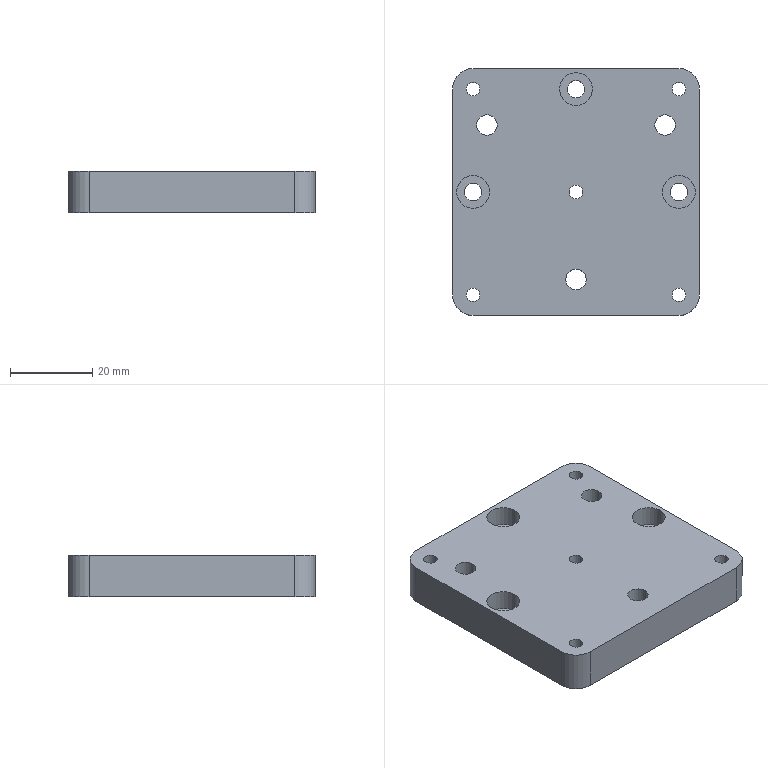Part | SolidWorks | features HoleWzd 3, Cut 1, Extrusion 1, Fillet 1, ICE 1 | 1 solid | 41 faces | box 60 x 60 x 10 mm | volume 33807 mm3 | cylinder 32 | plane 9 | commonest cylinder face diameters 3.3 x10 4.2 x6 5 x6 8 x6 10 x4
STEP:
#1=CARTESIAN_POINT('',(7.514,0.,0.));
#2=VERTEX_POINT('',#1);
#3=CARTESIAN_POINT('',(10.814,0.,0.));
#4=VERTEX_POINT('',#3);
#5=CARTESIAN_POINT('',(9.164,0.,0.));
#6=DIRECTION('',(0.,0.,1.));
#7=DIRECTION('',(1.,0.,0.));
#8=AXIS2_PLACEMENT_3D('',#5,#6,#7);
#9=CIRCLE('',#8,1.65);
#10=EDGE_CURVE('',#2,#4,#9,.T.);
#11=ORIENTED_EDGE('',*,*,#10,.F.);
#12=CARTESIAN_POINT('',(7.514,0.,10.));
#13=VERTEX_POINT('',#12);
#14=CARTESIAN_POINT('',(7.514,0.,10.));
#15=DIRECTION('',(0.,0.,1.));
#16=VECTOR('',#15,1000.);
#17=LINE('',#14,#16);
#18=EDGE_CURVE('',#2,#13,#17,.T.);
#19=ORIENTED_EDGE('',*,*,#18,.T.);
#20=CARTESIAN_POINT('',(10.814,0.,10.));
#21=VERTEX_POINT('',#20);
#22=CARTESIAN_POINT('',(9.164,0.,10.));
#23=DIRECTION('',(0.,0.,1.));
#24=DIRECTION('',(1.,0.,0.));
#25=AXIS2_PLACEMENT_3D('',#22,#23,#24);
#26=CIRCLE('',#25,1.65);
#27=EDGE_CURVE('',#13,#21,#26,.T.);
#28=ORIENTED_EDGE('',*,*,#27,.T.);
#29=CARTESIAN_POINT('',(10.814,0.,10.));
#30=DIRECTION('',(0.,0.,1.));
#31=VECTOR('',#30,1000.);
#32=LINE('',#29,#31);
#33=EDGE_CURVE('',#4,#21,#32,.T.);
#34=ORIENTED_EDGE('',*,*,#33,.F.);
#35=EDGE_LOOP('',(#11,#19,#28,#34));
#36=FACE_OUTER_BOUND('',#35,.T.);
#37=CARTESIAN_POINT('',(9.164,0.,10.));
#38=DIRECTION('',(0.,0.,1.));
#39=DIRECTION('',(1.,0.,0.));
#40=AXIS2_PLACEMENT_3D('',#37,#38,#39);
#41=CYLINDRICAL_SURFACE('',#40,1.65);
#42=ADVANCED_FACE('',(#36),#41,.F.);
#43=CARTESIAN_POINT('',(-17.486,-25.,0.));
#44=VERTEX_POINT('',#43);
#45=CARTESIAN_POINT('',(-14.186,-25.,0.));
#46=VERTEX_POINT('',#45);
#47=CARTESIAN_POINT('',(-15.836,-25.,0.));
#48=DIRECTION('',(0.,0.,1.));
#49=DIRECTION('',(1.,0.,0.));
#50=AXIS2_PLACEMENT_3D('',#47,#48,#49);
#51=CIRCLE('',#50,1.65);
#52=EDGE_CURVE('',#44,#46,#51,.T.);
#53=ORIENTED_EDGE('',*,*,#52,.F.);
#54=CARTESIAN_POINT('',(-17.486,-25.,10.));
#55=VERTEX_POINT('',#54);
#56=CARTESIAN_POINT('',(-17.486,-25.,10.));
#57=DIRECTION('',(0.,0.,1.));
#58=VECTOR('',#57,1000.);
#59=LINE('',#56,#58);
#60=EDGE_CURVE('',#44,#55,#59,.T.);
#61=ORIENTED_EDGE('',*,*,#60,.T.);
#62=CARTESIAN_POINT('',(-14.186,-25.,10.));
#63=VERTEX_POINT('',#62);
#64=CARTESIAN_POINT('',(-15.836,-25.,10.));
#65=DIRECTION('',(0.,0.,1.));
#66=DIRECTION('',(1.,0.,0.));
#67=AXIS2_PLACEMENT_3D('',#64,#65,#66);
#68=CIRCLE('',#67,1.65);
#69=EDGE_CURVE('',#55,#63,#68,.T.);
#70=ORIENTED_EDGE('',*,*,#69,.T.);
#71=CARTESIAN_POINT('',(-14.186,-25.,10.));
#72=DIRECTION('',(0.,0.,1.));
#73=VECTOR('',#72,1000.);
#74=LINE('',#71,#73);
#75=EDGE_CURVE('',#46,#63,#74,.T.);
#76=ORIENTED_EDGE('',*,*,#75,.F.);
#77=EDGE_LOOP('',(#53,#61,#70,#76));
#78=FACE_OUTER_BOUND('',#77,.T.);
#79=CARTESIAN_POINT('',(-15.836,-25.,10.));
#80=DIRECTION('',(0.,0.,1.));
#81=DIRECTION('',(1.,0.,0.));
#82=AXIS2_PLACEMENT_3D('',#79,#80,#81);
#83=CYLINDRICAL_SURFACE('',#82,1.65);
#84=ADVANCED_FACE('',(#78),#83,.F.);
#85=CARTESIAN_POINT('',(32.514,-25.,0.));
#86=VERTEX_POINT('',#85);
#87=CARTESIAN_POINT('',(35.814,-25.,0.));
#88=VERTEX_POINT('',#87);
#89=CARTESIAN_POINT('',(34.164,-25.,0.));
#90=DIRECTION('',(0.,0.,1.));
#91=DIRECTION('',(1.,0.,0.));
#92=AXIS2_PLACEMENT_3D('',#89,#90,#91);
#93=CIRCLE('',#92,1.65);
#94=EDGE_CURVE('',#86,#88,#93,.T.);
#95=ORIENTED_EDGE('',*,*,#94,.F.);
#96=CARTESIAN_POINT('',(32.514,-25.,10.));
#97=VERTEX_POINT('',#96);
#98=CARTESIAN_POINT('',(32.514,-25.,10.));
#99=DIRECTION('',(0.,0.,1.));
#100=VECTOR('',#99,1000.);
#101=LINE('',#98,#100);
#102=EDGE_CURVE('',#86,#97,#101,.T.);
#103=ORIENTED_EDGE('',*,*,#102,.T.);
#104=CARTESIAN_POINT('',(35.814,-25.,10.));
#105=VERTEX_POINT('',#104);
#106=CARTESIAN_POINT('',(34.164,-25.,10.));
#107=DIRECTION('',(0.,0.,1.));
#108=DIRECTION('',(1.,0.,0.));
#109=AXIS2_PLACEMENT_3D('',#106,#107,#108);
#110=CIRCLE('',#109,1.65);
#111=EDGE_CURVE('',#97,#105,#110,.T.);
#112=ORIENTED_EDGE('',*,*,#111,.T.);
#113=CARTESIAN_POINT('',(35.814,-25.,10.));
#114=DIRECTION('',(0.,0.,1.));
#115=VECTOR('',#114,1000.);
#116=LINE('',#113,#115);
#117=EDGE_CURVE('',#88,#105,#116,.T.);
#118=ORIENTED_EDGE('',*,*,#117,.F.);
#119=EDGE_LOOP('',(#95,#103,#112,#118));
#120=FACE_OUTER_BOUND('',#119,.T.);
#121=CARTESIAN_POINT('',(34.164,-25.,10.));
#122=DIRECTION('',(0.,0.,1.));
#123=DIRECTION('',(1.,0.,0.));
#124=AXIS2_PLACEMENT_3D('',#121,#122,#123);
#125=CYLINDRICAL_SURFACE('',#124,1.65);
#126=ADVANCED_FACE('',(#120),#125,.F.);
#127=CARTESIAN_POINT('',(32.514,25.,0.));
#128=VERTEX_POINT('',#127);
#129=CARTESIAN_POINT('',(35.814,25.,0.));
#130=VERTEX_POINT('',#129);
#131=CARTESIAN_POINT('',(34.164,25.,0.));
#132=DIRECTION('',(0.,0.,1.));
#133=DIRECTION('',(1.,0.,0.));
#134=AXIS2_PLACEMENT_3D('',#131,#132,#133);
#135=CIRCLE('',#134,1.65);
#136=EDGE_CURVE('',#128,#130,#135,.T.);
#137=ORIENTED_EDGE('',*,*,#136,.F.);
#138=CARTESIAN_POINT('',(32.514,25.,10.));
#139=VERTEX_POINT('',#138);
#140=CARTESIAN_POINT('',(32.514,25.,10.));
#141=DIRECTION('',(0.,0.,1.));
#142=VECTOR('',#141,1000.);
#143=LINE('',#140,#142);
#144=EDGE_CURVE('',#128,#139,#143,.T.);
#145=ORIENTED_EDGE('',*,*,#144,.T.);
#146=CARTESIAN_POINT('',(35.814,25.,10.));
#147=VERTEX_POINT('',#146);
#148=CARTESIAN_POINT('',(34.164,25.,10.));
#149=DIRECTION('',(0.,0.,1.));
#150=DIRECTION('',(1.,0.,0.));
#151=AXIS2_PLACEMENT_3D('',#148,#149,#150);
#152=CIRCLE('',#151,1.65);
#153=EDGE_CURVE('',#139,#147,#152,.T.);
#154=ORIENTED_EDGE('',*,*,#153,.T.);
#155=CARTESIAN_POINT('',(35.814,25.,10.));
#156=DIRECTION('',(0.,0.,1.));
#157=VECTOR('',#156,1000.);
#158=LINE('',#155,#157);
#159=EDGE_CURVE('',#130,#147,#158,.T.);
#160=ORIENTED_EDGE('',*,*,#159,.F.);
#161=EDGE_LOOP('',(#137,#145,#154,#160));
#162=FACE_OUTER_BOUND('',#161,.T.);
#163=CARTESIAN_POINT('',(34.164,25.,10.));
#164=DIRECTION('',(0.,0.,1.));
#165=DIRECTION('',(1.,0.,0.));
#166=AXIS2_PLACEMENT_3D('',#163,#164,#165);
#167=CYLINDRICAL_SURFACE('',#166,1.65);
#168=ADVANCED_FACE('',(#162),#167,.F.);
#169=CARTESIAN_POINT('',(-17.486,25.,0.));
#170=VERTEX_POINT('',#169);
#171=CARTESIAN_POINT('',(-14.186,25.,0.));
#172=VERTEX_POINT('',#171);
#173=CARTESIAN_POINT('',(-15.836,25.,0.));
#174=DIRECTION('',(0.,0.,1.));
#175=DIRECTION('',(1.,0.,0.));
#176=AXIS2_PLACEMENT_3D('',#173,#174,#175);
#177=CIRCLE('',#176,1.65);
#178=EDGE_CURVE('',#170,#172,#177,.T.);
#179=ORIENTED_EDGE('',*,*,#178,.F.);
#180=CARTESIAN_POINT('',(-17.486,25.,10.));
#181=VERTEX_POINT('',#180);
#182=CARTESIAN_POINT('',(-17.486,25.,10.));
#183=DIRECTION('',(0.,0.,1.));
#184=VECTOR('',#183,1000.);
#185=LINE('',#182,#184);
#186=EDGE_CURVE('',#170,#181,#185,.T.);
#187=ORIENTED_EDGE('',*,*,#186,.T.);
#188=CARTESIAN_POINT('',(-14.186,25.,10.));
#189=VERTEX_POINT('',#188);
#190=CARTESIAN_POINT('',(-15.836,25.,10.));
#191=DIRECTION('',(0.,0.,1.));
#192=DIRECTION('',(1.,0.,0.));
#193=AXIS2_PLACEMENT_3D('',#190,#191,#192);
#194=CIRCLE('',#193,1.65);
#195=EDGE_CURVE('',#181,#189,#194,.T.);
#196=ORIENTED_EDGE('',*,*,#195,.T.);
#197=CARTESIAN_POINT('',(-14.186,25.,10.));
#198=DIRECTION('',(0.,0.,1.));
#199=VECTOR('',#198,1000.);
#200=LINE('',#197,#199);
#201=EDGE_CURVE('',#172,#189,#200,.T.);
#202=ORIENTED_EDGE('',*,*,#201,.F.);
#203=EDGE_LOOP('',(#179,#187,#196,#202));
#204=FACE_OUTER_BOUND('',#203,.T.);
#205=CARTESIAN_POINT('',(-15.836,25.,10.));
#206=DIRECTION('',(0.,0.,1.));
#207=DIRECTION('',(1.,0.,0.));
#208=AXIS2_PLACEMENT_3D('',#205,#206,#207);
#209=CYLINDRICAL_SURFACE('',#208,1.65);
#210=ADVANCED_FACE('',(#204),#209,.F.);
#211=CARTESIAN_POINT('',(-19.836,0.,5.));
#212=VERTEX_POINT('',#211);
#213=CARTESIAN_POINT('',(-11.836,0.,5.));
#214=VERTEX_POINT('',#213);
#215=CARTESIAN_POINT('',(-15.836,0.,5.));
#216=DIRECTION('',(0.,0.,1.));
#217=DIRECTION('',(1.,0.,0.));
#218=AXIS2_PLACEMENT_3D('',#215,#216,#217);
#219=CIRCLE('',#218,4.);
#220=EDGE_CURVE('',#212,#214,#219,.T.);
#221=ORIENTED_EDGE('',*,*,#220,.F.);
#222=CARTESIAN_POINT('',(-19.836,0.,10.));
#223=VERTEX_POINT('',#222);
#224=CARTESIAN_POINT('',(-19.836,0.,5.));
#225=DIRECTION('',(0.,0.,1.));
#226=VECTOR('',#225,1000.);
#227=LINE('',#224,#226);
#228=EDGE_CURVE('',#212,#223,#227,.T.);
#229=ORIENTED_EDGE('',*,*,#228,.T.);
#230=CARTESIAN_POINT('',(-11.836,0.,10.));
#231=VERTEX_POINT('',#230);
#232=CARTESIAN_POINT('',(-15.836,0.,10.));
#233=DIRECTION('',(0.,0.,1.));
#234=DIRECTION('',(1.,0.,0.));
#235=AXIS2_PLACEMENT_3D('',#232,#233,#234);
#236=CIRCLE('',#235,4.);
#237=EDGE_CURVE('',#223,#231,#236,.T.);
#238=ORIENTED_EDGE('',*,*,#237,.T.);
#239=CARTESIAN_POINT('',(-11.836,0.,5.));
#240=DIRECTION('',(0.,0.,1.));
#241=VECTOR('',#240,1000.);
#242=LINE('',#239,#241);
#243=EDGE_CURVE('',#214,#231,#242,.T.);
#244=ORIENTED_EDGE('',*,*,#243,.F.);
#245=EDGE_LOOP('',(#221,#229,#238,#244));
#246=FACE_OUTER_BOUND('',#245,.T.);
#247=CARTESIAN_POINT('',(-15.836,0.,5.));
#248=DIRECTION('',(0.,0.,1.));
#249=DIRECTION('',(1.,0.,0.));
#250=AXIS2_PLACEMENT_3D('',#247,#248,#249);
#251=CYLINDRICAL_SURFACE('',#250,4.);
#252=ADVANCED_FACE('',(#246),#251,.F.);
#253=CARTESIAN_POINT('',(30.164,0.,5.));
#254=VERTEX_POINT('',#253);
#255=CARTESIAN_POINT('',(38.164,0.,5.));
#256=VERTEX_POINT('',#255);
#257=CARTESIAN_POINT('',(34.164,0.,5.));
#258=DIRECTION('',(0.,0.,1.));
#259=DIRECTION('',(1.,0.,0.));
#260=AXIS2_PLACEMENT_3D('',#257,#258,#259);
#261=CIRCLE('',#260,4.);
#262=EDGE_CURVE('',#254,#256,#261,.T.);
#263=ORIENTED_EDGE('',*,*,#262,.F.);
#264=CARTESIAN_POINT('',(30.164,0.,10.));
#265=VERTEX_POINT('',#264);
#266=CARTESIAN_POINT('',(30.164,0.,5.));
#267=DIRECTION('',(0.,0.,1.));
#268=VECTOR('',#267,1000.);
#269=LINE('',#266,#268);
#270=EDGE_CURVE('',#254,#265,#269,.T.);
#271=ORIENTED_EDGE('',*,*,#270,.T.);
#272=CARTESIAN_POINT('',(38.164,0.,10.));
#273=VERTEX_POINT('',#272);
#274=CARTESIAN_POINT('',(34.164,0.,10.));
#275=DIRECTION('',(0.,0.,1.));
#276=DIRECTION('',(1.,0.,0.));
#277=AXIS2_PLACEMENT_3D('',#274,#275,#276);
#278=CIRCLE('',#277,4.);
#279=EDGE_CURVE('',#265,#273,#278,.T.);
#280=ORIENTED_EDGE('',*,*,#279,.T.);
#281=CARTESIAN_POINT('',(38.164,0.,5.));
#282=DIRECTION('',(0.,0.,1.));
#283=VECTOR('',#282,1000.);
#284=LINE('',#281,#283);
#285=EDGE_CURVE('',#256,#273,#284,.T.);
#286=ORIENTED_EDGE('',*,*,#285,.F.);
#287=EDGE_LOOP('',(#263,#271,#280,#286));
#288=FACE_OUTER_BOUND('',#287,.T.);
#289=CARTESIAN_POINT('',(34.164,0.,5.));
#290=DIRECTION('',(0.,0.,1.));
#291=DIRECTION('',(1.,0.,0.));
#292=AXIS2_PLACEMENT_3D('',#289,#290,#291);
#293=CYLINDRICAL_SURFACE('',#292,4.);
#294=ADVANCED_FACE('',(#288),#293,.F.);
#295=CARTESIAN_POINT('',(5.164,25.,5.));
#296=VERTEX_POINT('',#295);
#297=CARTESIAN_POINT('',(13.164,25.,5.));
#298=VERTEX_POINT('',#297);
#299=CARTESIAN_POINT('',(9.164,25.,5.));
#300=DIRECTION('',(0.,0.,1.));
#301=DIRECTION('',(1.,0.,0.));
#302=AXIS2_PLACEMENT_3D('',#299,#300,#301);
#303=CIRCLE('',#302,4.);
#304=EDGE_CURVE('',#296,#298,#303,.T.);
#305=ORIENTED_EDGE('',*,*,#304,.F.);
#306=CARTESIAN_POINT('',(5.164,25.,10.));
#307=VERTEX_POINT('',#306);
#308=CARTESIAN_POINT('',(5.164,25.,5.));
#309=DIRECTION('',(0.,0.,1.));
#310=VECTOR('',#309,1000.);
#311=LINE('',#308,#310);
#312=EDGE_CURVE('',#296,#307,#311,.T.);
#313=ORIENTED_EDGE('',*,*,#312,.T.);
#314=CARTESIAN_POINT('',(13.164,25.,10.));
#315=VERTEX_POINT('',#314);
#316=CARTESIAN_POINT('',(9.164,25.,10.));
#317=DIRECTION('',(0.,0.,1.));
#318=DIRECTION('',(1.,0.,0.));
#319=AXIS2_PLACEMENT_3D('',#316,#317,#318);
#320=CIRCLE('',#319,4.);
#321=EDGE_CURVE('',#307,#315,#320,.T.);
#322=ORIENTED_EDGE('',*,*,#321,.T.);
#323=CARTESIAN_POINT('',(13.164,25.,5.));
#324=DIRECTION('',(0.,0.,1.));
#325=VECTOR('',#324,1000.);
#326=LINE('',#323,#325);
#327=EDGE_CURVE('',#298,#315,#326,.T.);
#328=ORIENTED_EDGE('',*,*,#327,.F.);
#329=EDGE_LOOP('',(#305,#313,#322,#328));
#330=FACE_OUTER_BOUND('',#329,.T.);
#331=CARTESIAN_POINT('',(9.164,25.,5.));
#332=DIRECTION('',(0.,0.,1.));
#333=DIRECTION('',(1.,0.,0.));
#334=AXIS2_PLACEMENT_3D('',#331,#332,#333);
#335=CYLINDRICAL_SURFACE('',#334,4.);
#336=ADVANCED_FACE('',(#330),#335,.F.);
#337=CARTESIAN_POINT('',(6.664,-21.25,0.));
#338=VERTEX_POINT('',#337);
#339=CARTESIAN_POINT('',(11.664,-21.25,0.));
#340=VERTEX_POINT('',#339);
#341=CARTESIAN_POINT('',(9.164,-21.25,0.));
#342=DIRECTION('',(0.,0.,1.));
#343=DIRECTION('',(1.,0.,0.));
#344=AXIS2_PLACEMENT_3D('',#341,#342,#343);
#345=CIRCLE('',#344,2.5);
#346=EDGE_CURVE('',#338,#340,#345,.T.);
#347=ORIENTED_EDGE('',*,*,#346,.F.);
#348=CARTESIAN_POINT('',(6.664,-21.25,10.));
#349=VERTEX_POINT('',#348);
#350=CARTESIAN_POINT('',(6.664,-21.25,10.));
#351=DIRECTION('',(0.,0.,1.));
#352=VECTOR('',#351,1000.);
#353=LINE('',#350,#352);
#354=EDGE_CURVE('',#338,#349,#353,.T.);
#355=ORIENTED_EDGE('',*,*,#354,.T.);
#356=CARTESIAN_POINT('',(11.664,-21.25,10.));
#357=VERTEX_POINT('',#356);
#358=CARTESIAN_POINT('',(9.164,-21.25,10.));
#359=DIRECTION('',(0.,0.,1.));
#360=DIRECTION('',(1.,0.,0.));
#361=AXIS2_PLACEMENT_3D('',#358,#359,#360);
#362=CIRCLE('',#361,2.5);
#363=EDGE_CURVE('',#349,#357,#362,.T.);
#364=ORIENTED_EDGE('',*,*,#363,.T.);
#365=CARTESIAN_POINT('',(11.664,-21.25,10.));
#366=DIRECTION('',(0.,0.,1.));
#367=VECTOR('',#366,1000.);
#368=LINE('',#365,#367);
#369=EDGE_CURVE('',#340,#357,#368,.T.);
#370=ORIENTED_EDGE('',*,*,#369,.F.);
#371=EDGE_LOOP('',(#347,#355,#364,#370));
#372=FACE_OUTER_BOUND('',#371,.T.);
#373=CARTESIAN_POINT('',(9.164,-21.25,10.));
#374=DIRECTION('',(0.,0.,1.));
#375=DIRECTION('',(1.,0.,0.));
#376=AXIS2_PLACEMENT_3D('',#373,#374,#375);
#377=CYLINDRICAL_SURFACE('',#376,2.5);
#378=ADVANCED_FACE('',(#372),#377,.F.);
#379=CARTESIAN_POINT('',(28.314,16.25,0.));
#380=VERTEX_POINT('',#379);
#381=CARTESIAN_POINT('',(33.314,16.25,0.));
#382=VERTEX_POINT('',#381);
#383=CARTESIAN_POINT('',(30.814,16.25,0.));
#384=DIRECTION('',(0.,0.,1.));
#385=DIRECTION('',(1.,0.,0.));
#386=AXIS2_PLACEMENT_3D('',#383,#384,#385);
#387=CIRCLE('',#386,2.5);
#388=EDGE_CURVE('',#380,#382,#387,.T.);
#389=ORIENTED_EDGE('',*,*,#388,.F.);
#390=CARTESIAN_POINT('',(28.314,16.25,10.));
#391=VERTEX_POINT('',#390);
#392=CARTESIAN_POINT('',(28.314,16.25,10.));
#393=DIRECTION('',(0.,0.,1.));
#394=VECTOR('',#393,1000.);
#395=LINE('',#392,#394);
#396=EDGE_CURVE('',#380,#391,#395,.T.);
#397=ORIENTED_EDGE('',*,*,#396,.T.);
#398=CARTESIAN_POINT('',(33.314,16.25,10.));
#399=VERTEX_POINT('',#398);
#400=CARTESIAN_POINT('',(30.814,16.25,10.));
#401=DIRECTION('',(0.,0.,1.));
#402=DIRECTION('',(1.,0.,0.));
#403=AXIS2_PLACEMENT_3D('',#400,#401,#402);
#404=CIRCLE('',#403,2.5);
#405=EDGE_CURVE('',#391,#399,#404,.T.);
#406=ORIENTED_EDGE('',*,*,#405,.T.);
#407=CARTESIAN_POINT('',(33.314,16.25,10.));
#408=DIRECTION('',(0.,0.,1.));
#409=VECTOR('',#408,1000.);
#410=LINE('',#407,#409);
#411=EDGE_CURVE('',#382,#399,#410,.T.);
#412=ORIENTED_EDGE('',*,*,#411,.F.);
#413=EDGE_LOOP('',(#389,#397,#406,#412));
#414=FACE_OUTER_BOUND('',#413,.T.);
#415=CARTESIAN_POINT('',(30.814,16.25,10.));
#416=DIRECTION('',(0.,0.,1.));
#417=DIRECTION('',(1.,0.,0.));
#418=AXIS2_PLACEMENT_3D('',#415,#416,#417);
#419=CYLINDRICAL_SURFACE('',#418,2.5);
#420=ADVANCED_FACE('',(#414),#419,.F.);
#421=CARTESIAN_POINT('',(-14.987,16.25,0.));
#422=VERTEX_POINT('',#421);
#423=CARTESIAN_POINT('',(-9.987,16.25,0.));
#424=VERTEX_POINT('',#423);
#425=CARTESIAN_POINT('',(-12.487,16.25,0.));
#426=DIRECTION('',(0.,0.,1.));
#427=DIRECTION('',(1.,0.,0.));
#428=AXIS2_PLACEMENT_3D('',#425,#426,#427);
#429=CIRCLE('',#428,2.5);
#430=EDGE_CURVE('',#422,#424,#429,.T.);
#431=ORIENTED_EDGE('',*,*,#430,.F.);
#432=CARTESIAN_POINT('',(-14.987,16.25,10.));
#433=VERTEX_POINT('',#432);
#434=CARTESIAN_POINT('',(-14.987,16.25,10.));
#435=DIRECTION('',(0.,0.,1.));
#436=VECTOR('',#435,1000.);
#437=LINE('',#434,#436);
#438=EDGE_CURVE('',#422,#433,#437,.T.);
#439=ORIENTED_EDGE('',*,*,#438,.T.);
#440=CARTESIAN_POINT('',(-9.987,16.25,10.));
#441=VERTEX_POINT('',#440);
#442=CARTESIAN_POINT('',(-12.487,16.25,10.));
#443=DIRECTION('',(0.,0.,1.));
#444=DIRECTION('',(1.,0.,0.));
#445=AXIS2_PLACEMENT_3D('',#442,#443,#444);
#446=CIRCLE('',#445,2.5);
#447=EDGE_CURVE('',#433,#441,#446,.T.);
#448=ORIENTED_EDGE('',*,*,#447,.T.);
#449=CARTESIAN_POINT('',(-9.987,16.25,10.));
#450=DIRECTION('',(0.,0.,1.));
#451=VECTOR('',#450,1000.);
#452=LINE('',#449,#451);
#453=EDGE_CURVE('',#424,#441,#452,.T.);
#454=ORIENTED_EDGE('',*,*,#453,.F.);
#455=EDGE_LOOP('',(#431,#439,#448,#454));
#456=FACE_OUTER_BOUND('',#455,.T.);
#457=CARTESIAN_POINT('',(-12.487,16.25,10.));
#458=DIRECTION('',(0.,0.,1.));
#459=DIRECTION('',(1.,0.,0.));
#460=AXIS2_PLACEMENT_3D('',#457,#458,#459);
#461=CYLINDRICAL_SURFACE('',#460,2.5);
#462=ADVANCED_FACE('',(#456),#461,.F.);
#463=CARTESIAN_POINT('',(7.064,25.,0.));
#464=VERTEX_POINT('',#463);
#465=CARTESIAN_POINT('',(11.264,25.,0.));
#466=VERTEX_POINT('',#465);
#467=CARTESIAN_POINT('',(9.164,25.,0.));
#468=DIRECTION('',(0.,0.,1.));
#469=DIRECTION('',(1.,0.,0.));
#470=AXIS2_PLACEMENT_3D('',#467,#468,#469);
#471=CIRCLE('',#470,2.1);
#472=EDGE_CURVE('',#464,#466,#471,.T.);
#473=ORIENTED_EDGE('',*,*,#472,.F.);
#474=CARTESIAN_POINT('',(7.064,25.,5.));
#475=VERTEX_POINT('',#474);
#476=CARTESIAN_POINT('',(7.064,25.,0.));
#477=DIRECTION('',(0.,0.,1.));
#478=VECTOR('',#477,1000.);
#479=LINE('',#476,#478);
#480=EDGE_CURVE('',#464,#475,#479,.T.);
#481=ORIENTED_EDGE('',*,*,#480,.T.);
#482=CARTESIAN_POINT('',(11.264,25.,5.));
#483=VERTEX_POINT('',#482);
#484=CARTESIAN_POINT('',(9.164,25.,5.));
#485=DIRECTION('',(0.,0.,-1.));
#486=DIRECTION('',(1.,0.,0.));
#487=AXIS2_PLACEMENT_3D('',#484,#485,#486);
#488=CIRCLE('',#487,2.1);
#489=EDGE_CURVE('',#483,#475,#488,.T.);
#490=ORIENTED_EDGE('',*,*,#489,.F.);
#491=CARTESIAN_POINT('',(11.264,25.,0.));
#492=DIRECTION('',(0.,0.,1.));
#493=VECTOR('',#492,1000.);
#494=LINE('',#491,#493);
#495=EDGE_CURVE('',#466,#483,#494,.T.);
#496=ORIENTED_EDGE('',*,*,#495,.F.);
#497=EDGE_LOOP('',(#473,#481,#490,#496));
#498=FACE_OUTER_BOUND('',#497,.T.);
#499=CARTESIAN_POINT('',(9.164,25.,0.));
#500=DIRECTION('',(0.,0.,1.));
#501=DIRECTION('',(1.,0.,0.));
#502=AXIS2_PLACEMENT_3D('',#499,#500,#501);
#503=CYLINDRICAL_SURFACE('',#502,2.1);
#504=ADVANCED_FACE('',(#498),#503,.F.);
#505=CARTESIAN_POINT('',(32.064,0.,0.));
#506=VERTEX_POINT('',#505);
#507=CARTESIAN_POINT('',(36.264,0.,0.));
#508=VERTEX_POINT('',#507);
#509=CARTESIAN_POINT('',(34.164,0.,0.));
#510=DIRECTION('',(0.,0.,1.));
#511=DIRECTION('',(1.,0.,0.));
#512=AXIS2_PLACEMENT_3D('',#509,#510,#511);
#513=CIRCLE('',#512,2.1);
#514=EDGE_CURVE('',#506,#508,#513,.T.);
#515=ORIENTED_EDGE('',*,*,#514,.F.);
#516=CARTESIAN_POINT('',(32.064,0.,5.));
#517=VERTEX_POINT('',#516);
#518=CARTESIAN_POINT('',(32.064,0.,0.));
#519=DIRECTION('',(0.,0.,1.));
#520=VECTOR('',#519,1000.);
#521=LINE('',#518,#520);
#522=EDGE_CURVE('',#506,#517,#521,.T.);
#523=ORIENTED_EDGE('',*,*,#522,.T.);
#524=CARTESIAN_POINT('',(36.264,0.,5.));
#525=VERTEX_POINT('',#524);
#526=CARTESIAN_POINT('',(34.164,0.,5.));
#527=DIRECTION('',(0.,0.,-1.));
#528=DIRECTION('',(1.,0.,0.));
#529=AXIS2_PLACEMENT_3D('',#526,#527,#528);
#530=CIRCLE('',#529,2.1);
#531=EDGE_CURVE('',#525,#517,#530,.T.);
#532=ORIENTED_EDGE('',*,*,#531,.F.);
#533=CARTESIAN_POINT('',(36.264,0.,0.));
#534=DIRECTION('',(0.,0.,1.));
#535=VECTOR('',#534,1000.);
#536=LINE('',#533,#535);
#537=EDGE_CURVE('',#508,#525,#536,.T.);
#538=ORIENTED_EDGE('',*,*,#537,.F.);
#539=EDGE_LOOP('',(#515,#523,#532,#538));
#540=FACE_OUTER_BOUND('',#539,.T.);
#541=CARTESIAN_POINT('',(34.164,0.,0.));
#542=DIRECTION('',(0.,0.,1.));
#543=DIRECTION('',(1.,0.,0.));
#544=AXIS2_PLACEMENT_3D('',#541,#542,#543);
#545=CYLINDRICAL_SURFACE('',#544,2.1);
#546=ADVANCED_FACE('',(#540),#545,.F.);
#547=CARTESIAN_POINT('',(-17.936,0.,0.));
#548=VERTEX_POINT('',#547);
#549=CARTESIAN_POINT('',(-13.736,0.,0.));
#550=VERTEX_POINT('',#549);
#551=CARTESIAN_POINT('',(-15.836,0.,0.));
#552=DIRECTION('',(0.,0.,1.));
#553=DIRECTION('',(1.,0.,0.));
#554=AXIS2_PLACEMENT_3D('',#551,#552,#553);
#555=CIRCLE('',#554,2.1);
#556=EDGE_CURVE('',#548,#550,#555,.T.);
#557=ORIENTED_EDGE('',*,*,#556,.F.);
#558=CARTESIAN_POINT('',(-17.936,0.,5.));
#559=VERTEX_POINT('',#558);
#560=CARTESIAN_POINT('',(-17.936,0.,0.));
#561=DIRECTION('',(0.,0.,1.));
#562=VECTOR('',#561,1000.);
#563=LINE('',#560,#562);
#564=EDGE_CURVE('',#548,#559,#563,.T.);
#565=ORIENTED_EDGE('',*,*,#564,.T.);
#566=CARTESIAN_POINT('',(-13.736,0.,5.));
#567=VERTEX_POINT('',#566);
#568=CARTESIAN_POINT('',(-15.836,0.,5.));
#569=DIRECTION('',(0.,0.,-1.));
#570=DIRECTION('',(1.,0.,0.));
#571=AXIS2_PLACEMENT_3D('',#568,#569,#570);
#572=CIRCLE('',#571,2.1);
#573=EDGE_CURVE('',#567,#559,#572,.T.);
#574=ORIENTED_EDGE('',*,*,#573,.F.);
#575=CARTESIAN_POINT('',(-13.736,0.,0.));
#576=DIRECTION('',(0.,0.,1.));
#577=VECTOR('',#576,1000.);
#578=LINE('',#575,#577);
#579=EDGE_CURVE('',#550,#567,#578,.T.);
#580=ORIENTED_EDGE('',*,*,#579,.F.);
#581=EDGE_LOOP('',(#557,#565,#574,#580));
#582=FACE_OUTER_BOUND('',#581,.T.);
#583=CARTESIAN_POINT('',(-15.836,0.,0.));
#584=DIRECTION('',(0.,0.,1.));
#585=DIRECTION('',(1.,0.,0.));
#586=AXIS2_PLACEMENT_3D('',#583,#584,#585);
#587=CYLINDRICAL_SURFACE('',#586,2.1);
#588=ADVANCED_FACE('',(#582),#587,.F.);
#589=ORIENTED_EDGE('',*,*,#564,.F.);
#590=CARTESIAN_POINT('',(-15.836,0.,0.));
#591=DIRECTION('',(0.,0.,1.));
#592=DIRECTION('',(1.,0.,0.));
#593=AXIS2_PLACEMENT_3D('',#590,#591,#592);
#594=CIRCLE('',#593,2.1);
#595=EDGE_CURVE('',#550,#548,#594,.T.);
#596=ORIENTED_EDGE('',*,*,#595,.F.);
#597=ORIENTED_EDGE('',*,*,#579,.T.);
#598=CARTESIAN_POINT('',(-15.836,0.,5.));
#599=DIRECTION('',(0.,0.,-1.));
#600=DIRECTION('',(1.,0.,0.));
#601=AXIS2_PLACEMENT_3D('',#598,#599,#600);
#602=CIRCLE('',#601,2.1);
#603=EDGE_CURVE('',#559,#567,#602,.T.);
#604=ORIENTED_EDGE('',*,*,#603,.F.);
#605=EDGE_LOOP('',(#589,#596,#597,#604));
#606=FACE_OUTER_BOUND('',#605,.T.);
#607=CARTESIAN_POINT('',(-15.836,0.,0.));
#608=DIRECTION('',(0.,0.,1.));
#609=DIRECTION('',(1.,0.,0.));
#610=AXIS2_PLACEMENT_3D('',#607,#608,#609);
#611=CYLINDRICAL_SURFACE('',#610,2.1);
#612=ADVANCED_FACE('',(#606),#611,.F.);
#613=ORIENTED_EDGE('',*,*,#522,.F.);
#614=CARTESIAN_POINT('',(34.164,0.,0.));
#615=DIRECTION('',(0.,0.,1.));
#616=DIRECTION('',(1.,0.,0.));
#617=AXIS2_PLACEMENT_3D('',#614,#615,#616);
#618=CIRCLE('',#617,2.1);
#619=EDGE_CURVE('',#508,#506,#618,.T.);
#620=ORIENTED_EDGE('',*,*,#619,.F.);
#621=ORIENTED_EDGE('',*,*,#537,.T.);
#622=CARTESIAN_POINT('',(34.164,0.,5.));
#623=DIRECTION('',(0.,0.,-1.));
#624=DIRECTION('',(1.,0.,0.));
#625=AXIS2_PLACEMENT_3D('',#622,#623,#624);
#626=CIRCLE('',#625,2.1);
#627=EDGE_CURVE('',#517,#525,#626,.T.);
#628=ORIENTED_EDGE('',*,*,#627,.F.);
#629=EDGE_LOOP('',(#613,#620,#621,#628));
#630=FACE_OUTER_BOUND('',#629,.T.);
#631=CARTESIAN_POINT('',(34.164,0.,0.));
#632=DIRECTION('',(0.,0.,1.));
#633=DIRECTION('',(1.,0.,0.));
#634=AXIS2_PLACEMENT_3D('',#631,#632,#633);
#635=CYLINDRICAL_SURFACE('',#634,2.1);
#636=ADVANCED_FACE('',(#630),#635,.F.);
#637=ORIENTED_EDGE('',*,*,#480,.F.);
#638=CARTESIAN_POINT('',(9.164,25.,0.));
#639=DIRECTION('',(0.,0.,1.));
#640=DIRECTION('',(1.,0.,0.));
#641=AXIS2_PLACEMENT_3D('',#638,#639,#640);
#642=CIRCLE('',#641,2.1);
#643=EDGE_CURVE('',#466,#464,#642,.T.);
#644=ORIENTED_EDGE('',*,*,#643,.F.);
#645=ORIENTED_EDGE('',*,*,#495,.T.);
#646=CARTESIAN_POINT('',(9.164,25.,5.));
#647=DIRECTION('',(0.,0.,-1.));
#648=DIRECTION('',(1.,0.,0.));
#649=AXIS2_PLACEMENT_3D('',#646,#647,#648);
#650=CIRCLE('',#649,2.1);
#651=EDGE_CURVE('',#475,#483,#650,.T.);
#652=ORIENTED_EDGE('',*,*,#651,.F.);
#653=EDGE_LOOP('',(#637,#644,#645,#652));
#654=FACE_OUTER_BOUND('',#653,.T.);
#655=CARTESIAN_POINT('',(9.164,25.,0.));
#656=DIRECTION('',(0.,0.,1.));
#657=DIRECTION('',(1.,0.,0.));
#658=AXIS2_PLACEMENT_3D('',#655,#656,#657);
#659=CYLINDRICAL_SURFACE('',#658,2.1);
#660=ADVANCED_FACE('',(#654),#659,.F.);
#661=CARTESIAN_POINT('',(-20.836,25.,10.));
#662=VERTEX_POINT('',#661);
#663=CARTESIAN_POINT('',(-20.836,-25.,10.));
#664=VERTEX_POINT('',#663);
#665=CARTESIAN_POINT('',(-20.836,-30.,10.));
#666=DIRECTION('',(0.,-1.,0.));
#667=VECTOR('',#666,1000.);
#668=LINE('',#665,#667);
#669=EDGE_CURVE('',#662,#664,#668,.T.);
#670=ORIENTED_EDGE('',*,*,#669,.F.);
#671=CARTESIAN_POINT('',(-20.836,25.,0.));
#672=VERTEX_POINT('',#671);
#673=CARTESIAN_POINT('',(-20.836,25.,10.));
#674=DIRECTION('',(0.,0.,-1.));
#675=VECTOR('',#674,1000.);
#676=LINE('',#673,#675);
#677=EDGE_CURVE('',#662,#672,#676,.T.);
#678=ORIENTED_EDGE('',*,*,#677,.T.);
#679=CARTESIAN_POINT('',(-20.836,-25.,0.));
#680=VERTEX_POINT('',#679);
#681=CARTESIAN_POINT('',(-20.836,-30.,0.));
#682=DIRECTION('',(0.,-1.,0.));
#683=VECTOR('',#682,1000.);
#684=LINE('',#681,#683);
#685=EDGE_CURVE('',#672,#680,#684,.T.);
#686=ORIENTED_EDGE('',*,*,#685,.T.);
#687=CARTESIAN_POINT('',(-20.836,-25.,10.));
#688=DIRECTION('',(0.,0.,1.));
#689=VECTOR('',#688,1000.);
#690=LINE('',#687,#689);
#691=EDGE_CURVE('',#680,#664,#690,.T.);
#692=ORIENTED_EDGE('',*,*,#691,.T.);
#693=EDGE_LOOP('',(#670,#678,#686,#692));
#694=FACE_OUTER_BOUND('',#693,.T.);
#695=CARTESIAN_POINT('',(-20.836,-30.,10.));
#696=DIRECTION('',(1.,0.,0.));
#697=DIRECTION('',(0.,0.,-1.));
#698=AXIS2_PLACEMENT_3D('',#695,#696,#697);
#699=PLANE('',#698);
#700=ADVANCED_FACE('',(#694),#699,.F.);
#701=CARTESIAN_POINT('',(-15.836,-30.,0.));
#702=VERTEX_POINT('',#701);
#703=CARTESIAN_POINT('',(34.164,-30.,0.));
#704=VERTEX_POINT('',#703);
#705=CARTESIAN_POINT('',(39.164,-30.,0.));
#706=DIRECTION('',(1.,0.,0.));
#707=VECTOR('',#706,1000.);
#708=LINE('',#705,#707);
#709=EDGE_CURVE('',#702,#704,#708,.T.);
#710=ORIENTED_EDGE('',*,*,#709,.T.);
#711=CARTESIAN_POINT('',(34.164,-30.,10.));
#712=VERTEX_POINT('',#711);
#713=CARTESIAN_POINT('',(34.164,-30.,10.));
#714=DIRECTION('',(0.,0.,1.));
#715=VECTOR('',#714,1000.);
#716=LINE('',#713,#715);
#717=EDGE_CURVE('',#704,#712,#716,.T.);
#718=ORIENTED_EDGE('',*,*,#717,.T.);
#719=CARTESIAN_POINT('',(-15.836,-30.,10.));
#720=VERTEX_POINT('',#719);
#721=CARTESIAN_POINT('',(39.164,-30.,10.));
#722=DIRECTION('',(1.,0.,0.));
#723=VECTOR('',#722,1000.);
#724=LINE('',#721,#723);
#725=EDGE_CURVE('',#720,#712,#724,.T.);
#726=ORIENTED_EDGE('',*,*,#725,.F.);
#727=CARTESIAN_POINT('',(-15.836,-30.,10.));
#728=DIRECTION('',(0.,0.,-1.));
#729=VECTOR('',#728,1000.);
#730=LINE('',#727,#729);
#731=EDGE_CURVE('',#720,#702,#730,.T.);
#732=ORIENTED_EDGE('',*,*,#731,.T.);
#733=EDGE_LOOP('',(#710,#718,#726,#732));
#734=FACE_OUTER_BOUND('',#733,.T.);
#735=CARTESIAN_POINT('',(39.164,-30.,10.));
#736=DIRECTION('',(0.,1.,0.));
#737=DIRECTION('',(-1.,0.,0.));
#738=AXIS2_PLACEMENT_3D('',#735,#736,#737);
#739=PLANE('',#738);
#740=ADVANCED_FACE('',(#734),#739,.F.);
#741=CARTESIAN_POINT('',(39.164,-25.,0.));
#742=VERTEX_POINT('',#741);
#743=CARTESIAN_POINT('',(39.164,25.,0.));
#744=VERTEX_POINT('',#743);
#745=CARTESIAN_POINT('',(39.164,-30.,0.));
#746=DIRECTION('',(0.,1.,0.));
#747=VECTOR('',#746,1000.);
#748=LINE('',#745,#747);
#749=EDGE_CURVE('',#742,#744,#748,.T.);
#750=ORIENTED_EDGE('',*,*,#749,.T.);
#751=CARTESIAN_POINT('',(39.164,25.,10.));
#752=VERTEX_POINT('',#751);
#753=CARTESIAN_POINT('',(39.164,25.,10.));
#754=DIRECTION('',(0.,0.,1.));
#755=VECTOR('',#754,1000.);
#756=LINE('',#753,#755);
#757=EDGE_CURVE('',#744,#752,#756,.T.);
#758=ORIENTED_EDGE('',*,*,#757,.T.);
#759=CARTESIAN_POINT('',(39.164,-25.,10.));
#760=VERTEX_POINT('',#759);
#761=CARTESIAN_POINT('',(39.164,-30.,10.));
#762=DIRECTION('',(0.,1.,0.));
#763=VECTOR('',#762,1000.);
#764=LINE('',#761,#763);
#765=EDGE_CURVE('',#760,#752,#764,.T.);
#766=ORIENTED_EDGE('',*,*,#765,.F.);
#767=CARTESIAN_POINT('',(39.164,-25.,10.));
#768=DIRECTION('',(0.,0.,-1.));
#769=VECTOR('',#768,1000.);
#770=LINE('',#767,#769);
#771=EDGE_CURVE('',#760,#742,#770,.T.);
#772=ORIENTED_EDGE('',*,*,#771,.T.);
#773=EDGE_LOOP('',(#750,#758,#766,#772));
#774=FACE_OUTER_BOUND('',#773,.T.);
#775=CARTESIAN_POINT('',(39.164,-30.,10.));
#776=DIRECTION('',(-1.,0.,0.));
#777=DIRECTION('',(0.,0.,1.));
#778=AXIS2_PLACEMENT_3D('',#775,#776,#777);
#779=PLANE('',#778);
#780=ADVANCED_FACE('',(#774),#779,.F.);
#781=CARTESIAN_POINT('',(34.164,30.,0.));
#782=VERTEX_POINT('',#781);
#783=CARTESIAN_POINT('',(-15.836,30.,0.));
#784=VERTEX_POINT('',#783);
#785=CARTESIAN_POINT('',(39.164,30.,0.));
#786=DIRECTION('',(-1.,0.,0.));
#787=VECTOR('',#786,1000.);
#788=LINE('',#785,#787);
#789=EDGE_CURVE('',#782,#784,#788,.T.);
#790=ORIENTED_EDGE('',*,*,#789,.T.);
#791=CARTESIAN_POINT('',(-15.836,30.,10.));
#792=VERTEX_POINT('',#791);
#793=CARTESIAN_POINT('',(-15.836,30.,10.));
#794=DIRECTION('',(0.,0.,1.));
#795=VECTOR('',#794,1000.);
#796=LINE('',#793,#795);
#797=EDGE_CURVE('',#784,#792,#796,.T.);
#798=ORIENTED_EDGE('',*,*,#797,.T.);
#799=CARTESIAN_POINT('',(34.164,30.,10.));
#800=VERTEX_POINT('',#799);
#801=CARTESIAN_POINT('',(39.164,30.,10.));
#802=DIRECTION('',(-1.,0.,0.));
#803=VECTOR('',#802,1000.);
#804=LINE('',#801,#803);
#805=EDGE_CURVE('',#800,#792,#804,.T.);
#806=ORIENTED_EDGE('',*,*,#805,.F.);
#807=CARTESIAN_POINT('',(34.164,30.,10.));
#808=DIRECTION('',(0.,0.,-1.));
#809=VECTOR('',#808,1000.);
#810=LINE('',#807,#809);
#811=EDGE_CURVE('',#800,#782,#810,.T.);
#812=ORIENTED_EDGE('',*,*,#811,.T.);
#813=EDGE_LOOP('',(#790,#798,#806,#812));
#814=FACE_OUTER_BOUND('',#813,.T.);
#815=CARTESIAN_POINT('',(39.164,30.,10.));
#816=DIRECTION('',(0.,-1.,0.));
#817=DIRECTION('',(1.,0.,0.));
#818=AXIS2_PLACEMENT_3D('',#815,#816,#817);
#819=PLANE('',#818);
#820=ADVANCED_FACE('',(#814),#819,.F.);
#821=CARTESIAN_POINT('',(9.164,0.,10.));
#822=DIRECTION('',(0.,0.,1.));
#823=DIRECTION('',(1.,0.,0.));
#824=AXIS2_PLACEMENT_3D('',#821,#822,#823);
#825=CIRCLE('',#824,1.65);
#826=EDGE_CURVE('',#21,#13,#825,.T.);
#827=ORIENTED_EDGE('',*,*,#826,.F.);
#828=ORIENTED_EDGE('',*,*,#27,.F.);
#829=EDGE_LOOP('',(#827,#828));
#830=FACE_BOUND('',#829,.T.);
#831=CARTESIAN_POINT('',(-15.836,-25.,10.));
#832=DIRECTION('',(0.,0.,1.));
#833=DIRECTION('',(1.,0.,0.));
#834=AXIS2_PLACEMENT_3D('',#831,#832,#833);
#835=CIRCLE('',#834,1.65);
#836=EDGE_CURVE('',#63,#55,#835,.T.);
#837=ORIENTED_EDGE('',*,*,#836,.F.);
#838=ORIENTED_EDGE('',*,*,#69,.F.);
#839=EDGE_LOOP('',(#837,#838));
#840=FACE_BOUND('',#839,.T.);
#841=CARTESIAN_POINT('',(34.164,-25.,10.));
#842=DIRECTION('',(0.,0.,1.));
#843=DIRECTION('',(1.,0.,0.));
#844=AXIS2_PLACEMENT_3D('',#841,#842,#843);
#845=CIRCLE('',#844,1.65);
#846=EDGE_CURVE('',#105,#97,#845,.T.);
#847=ORIENTED_EDGE('',*,*,#846,.F.);
#848=ORIENTED_EDGE('',*,*,#111,.F.);
#849=EDGE_LOOP('',(#847,#848));
#850=FACE_BOUND('',#849,.T.);
#851=CARTESIAN_POINT('',(34.164,25.,10.));
#852=DIRECTION('',(0.,0.,1.));
#853=DIRECTION('',(1.,0.,0.));
#854=AXIS2_PLACEMENT_3D('',#851,#852,#853);
#855=CIRCLE('',#854,1.65);
#856=EDGE_CURVE('',#147,#139,#855,.T.);
#857=ORIENTED_EDGE('',*,*,#856,.F.);
#858=ORIENTED_EDGE('',*,*,#153,.F.);
#859=EDGE_LOOP('',(#857,#858));
#860=FACE_BOUND('',#859,.T.);
#861=CARTESIAN_POINT('',(-15.836,25.,10.));
#862=DIRECTION('',(0.,0.,1.));
#863=DIRECTION('',(1.,0.,0.));
#864=AXIS2_PLACEMENT_3D('',#861,#862,#863);
#865=CIRCLE('',#864,1.65);
#866=EDGE_CURVE('',#189,#181,#865,.T.);
#867=ORIENTED_EDGE('',*,*,#866,.F.);
#868=ORIENTED_EDGE('',*,*,#195,.F.);
#869=EDGE_LOOP('',(#867,#868));
#870=FACE_BOUND('',#869,.T.);
#871=CARTESIAN_POINT('',(-15.836,0.,10.));
#872=DIRECTION('',(0.,0.,1.));
#873=DIRECTION('',(1.,0.,0.));
#874=AXIS2_PLACEMENT_3D('',#871,#872,#873);
#875=CIRCLE('',#874,4.);
#876=EDGE_CURVE('',#231,#223,#875,.T.);
#877=ORIENTED_EDGE('',*,*,#876,.F.);
#878=ORIENTED_EDGE('',*,*,#237,.F.);
#879=EDGE_LOOP('',(#877,#878));
#880=FACE_BOUND('',#879,.T.);
#881=CARTESIAN_POINT('',(9.164,25.,10.));
#882=DIRECTION('',(0.,0.,1.));
#883=DIRECTION('',(1.,0.,0.));
#884=AXIS2_PLACEMENT_3D('',#881,#882,#883);
#885=CIRCLE('',#884,4.);
#886=EDGE_CURVE('',#315,#307,#885,.T.);
#887=ORIENTED_EDGE('',*,*,#886,.F.);
#888=ORIENTED_EDGE('',*,*,#321,.F.);
#889=EDGE_LOOP('',(#887,#888));
#890=FACE_BOUND('',#889,.T.);
#891=CARTESIAN_POINT('',(34.164,0.,10.));
#892=DIRECTION('',(0.,0.,1.));
#893=DIRECTION('',(1.,0.,0.));
#894=AXIS2_PLACEMENT_3D('',#891,#892,#893);
#895=CIRCLE('',#894,4.);
#896=EDGE_CURVE('',#273,#265,#895,.T.);
#897=ORIENTED_EDGE('',*,*,#896,.F.);
#898=ORIENTED_EDGE('',*,*,#279,.F.);
#899=EDGE_LOOP('',(#897,#898));
#900=FACE_BOUND('',#899,.T.);
#901=CARTESIAN_POINT('',(9.164,-21.25,10.));
#902=DIRECTION('',(0.,0.,1.));
#903=DIRECTION('',(1.,0.,0.));
#904=AXIS2_PLACEMENT_3D('',#901,#902,#903);
#905=CIRCLE('',#904,2.5);
#906=EDGE_CURVE('',#357,#349,#905,.T.);
#907=ORIENTED_EDGE('',*,*,#906,.F.);
#908=ORIENTED_EDGE('',*,*,#363,.F.);
#909=EDGE_LOOP('',(#907,#908));
#910=FACE_BOUND('',#909,.T.);
#911=CARTESIAN_POINT('',(30.814,16.25,10.));
#912=DIRECTION('',(0.,0.,1.));
#913=DIRECTION('',(1.,0.,0.));
#914=AXIS2_PLACEMENT_3D('',#911,#912,#913);
#915=CIRCLE('',#914,2.5);
#916=EDGE_CURVE('',#399,#391,#915,.T.);
#917=ORIENTED_EDGE('',*,*,#916,.F.);
#918=ORIENTED_EDGE('',*,*,#405,.F.);
#919=EDGE_LOOP('',(#917,#918));
#920=FACE_BOUND('',#919,.T.);
#921=CARTESIAN_POINT('',(-12.487,16.25,10.));
#922=DIRECTION('',(0.,0.,1.));
#923=DIRECTION('',(1.,0.,0.));
#924=AXIS2_PLACEMENT_3D('',#921,#922,#923);
#925=CIRCLE('',#924,2.5);
#926=EDGE_CURVE('',#441,#433,#925,.T.);
#927=ORIENTED_EDGE('',*,*,#926,.F.);
#928=ORIENTED_EDGE('',*,*,#447,.F.);
#929=EDGE_LOOP('',(#927,#928));
#930=FACE_BOUND('',#929,.T.);
#931=ORIENTED_EDGE('',*,*,#805,.T.);
#932=CARTESIAN_POINT('',(-15.836,25.,10.));
#933=DIRECTION('',(0.,0.,1.));
#934=DIRECTION('',(1.,0.,0.));
#935=AXIS2_PLACEMENT_3D('',#932,#933,#934);
#936=CIRCLE('',#935,5.);
#937=EDGE_CURVE('',#792,#662,#936,.T.);
#938=ORIENTED_EDGE('',*,*,#937,.T.);
#939=ORIENTED_EDGE('',*,*,#669,.T.);
#940=CARTESIAN_POINT('',(-15.836,-25.,10.));
#941=DIRECTION('',(0.,0.,1.));
#942=DIRECTION('',(1.,0.,0.));
#943=AXIS2_PLACEMENT_3D('',#940,#941,#942);
#944=CIRCLE('',#943,5.);
#945=EDGE_CURVE('',#664,#720,#944,.T.);
#946=ORIENTED_EDGE('',*,*,#945,.T.);
#947=ORIENTED_EDGE('',*,*,#725,.T.);
#948=CARTESIAN_POINT('',(34.164,-25.,10.));
#949=DIRECTION('',(0.,0.,1.));
#950=DIRECTION('',(1.,0.,0.));
#951=AXIS2_PLACEMENT_3D('',#948,#949,#950);
#952=CIRCLE('',#951,5.);
#953=EDGE_CURVE('',#712,#760,#952,.T.);
#954=ORIENTED_EDGE('',*,*,#953,.T.);
#955=ORIENTED_EDGE('',*,*,#765,.T.);
#956=CARTESIAN_POINT('',(34.164,25.,10.));
#957=DIRECTION('',(0.,0.,1.));
#958=DIRECTION('',(1.,0.,0.));
#959=AXIS2_PLACEMENT_3D('',#956,#957,#958);
#960=CIRCLE('',#959,5.);
#961=EDGE_CURVE('',#752,#800,#960,.T.);
#962=ORIENTED_EDGE('',*,*,#961,.T.);
#963=EDGE_LOOP('',(#931,#938,#939,#946,#947,#954,#955,#962));
#964=FACE_OUTER_BOUND('',#963,.T.);
#965=CARTESIAN_POINT('',(0.,0.,10.));
#966=DIRECTION('',(0.,0.,1.));
#967=DIRECTION('',(1.,0.,0.));
#968=AXIS2_PLACEMENT_3D('',#965,#966,#967);
#969=PLANE('',#968);
#970=ADVANCED_FACE('',(#830,#840,#850,#860,#870,#880,#890,#900,#910,#920,#930,#964),#969,.T.);
#971=CARTESIAN_POINT('',(9.164,0.,0.));
#972=DIRECTION('',(0.,0.,1.));
#973=DIRECTION('',(1.,0.,0.));
#974=AXIS2_PLACEMENT_3D('',#971,#972,#973);
#975=CIRCLE('',#974,1.65);
#976=EDGE_CURVE('',#4,#2,#975,.T.);
#977=ORIENTED_EDGE('',*,*,#976,.T.);
#978=ORIENTED_EDGE('',*,*,#10,.T.);
#979=EDGE_LOOP('',(#977,#978));
#980=FACE_BOUND('',#979,.T.);
#981=CARTESIAN_POINT('',(-15.836,-25.,0.));
#982=DIRECTION('',(0.,0.,1.));
#983=DIRECTION('',(1.,0.,0.));
#984=AXIS2_PLACEMENT_3D('',#981,#982,#983);
#985=CIRCLE('',#984,1.65);
#986=EDGE_CURVE('',#46,#44,#985,.T.);
#987=ORIENTED_EDGE('',*,*,#986,.T.);
#988=ORIENTED_EDGE('',*,*,#52,.T.);
#989=EDGE_LOOP('',(#987,#988));
#990=FACE_BOUND('',#989,.T.);
#991=CARTESIAN_POINT('',(34.164,-25.,0.));
#992=DIRECTION('',(0.,0.,1.));
#993=DIRECTION('',(1.,0.,0.));
#994=AXIS2_PLACEMENT_3D('',#991,#992,#993);
#995=CIRCLE('',#994,1.65);
#996=EDGE_CURVE('',#88,#86,#995,.T.);
#997=ORIENTED_EDGE('',*,*,#996,.T.);
#998=ORIENTED_EDGE('',*,*,#94,.T.);
#999=EDGE_LOOP('',(#997,#998));
#1000=FACE_BOUND('',#999,.T.);
#1001=CARTESIAN_POINT('',(34.164,25.,0.));
#1002=DIRECTION('',(0.,0.,1.));
#1003=DIRECTION('',(1.,0.,0.));
#1004=AXIS2_PLACEMENT_3D('',#1001,#1002,#1003);
#1005=CIRCLE('',#1004,1.65);
#1006=EDGE_CURVE('',#130,#128,#1005,.T.);
#1007=ORIENTED_EDGE('',*,*,#1006,.T.);
#1008=ORIENTED_EDGE('',*,*,#136,.T.);
#1009=EDGE_LOOP('',(#1007,#1008));
#1010=FACE_BOUND('',#1009,.T.);
#1011=CARTESIAN_POINT('',(-15.836,25.,0.));
#1012=DIRECTION('',(0.,0.,1.));
#1013=DIRECTION('',(1.,0.,0.));
#1014=AXIS2_PLACEMENT_3D('',#1011,#1012,#1013);
#1015=CIRCLE('',#1014,1.65);
#1016=EDGE_CURVE('',#172,#170,#1015,.T.);
#1017=ORIENTED_EDGE('',*,*,#1016,.T.);
#1018=ORIENTED_EDGE('',*,*,#178,.T.);
#1019=EDGE_LOOP('',(#1017,#1018));
#1020=FACE_BOUND('',#1019,.T.);
#1021=ORIENTED_EDGE('',*,*,#643,.T.);
#1022=ORIENTED_EDGE('',*,*,#472,.T.);
#1023=EDGE_LOOP('',(#1021,#1022));
#1024=FACE_BOUND('',#1023,.T.);
#1025=ORIENTED_EDGE('',*,*,#619,.T.);
#1026=ORIENTED_EDGE('',*,*,#514,.T.);
#1027=EDGE_LOOP('',(#1025,#1026));
#1028=FACE_BOUND('',#1027,.T.);
#1029=ORIENTED_EDGE('',*,*,#595,.T.);
#1030=ORIENTED_EDGE('',*,*,#556,.T.);
#1031=EDGE_LOOP('',(#1029,#1030));
#1032=FACE_BOUND('',#1031,.T.);
#1033=CARTESIAN_POINT('',(9.164,-21.25,0.));
#1034=DIRECTION('',(0.,0.,1.));
#1035=DIRECTION('',(1.,0.,0.));
#1036=AXIS2_PLACEMENT_3D('',#1033,#1034,#1035);
#1037=CIRCLE('',#1036,2.5);
#1038=EDGE_CURVE('',#340,#338,#1037,.T.);
#1039=ORIENTED_EDGE('',*,*,#1038,.T.);
#1040=ORIENTED_EDGE('',*,*,#346,.T.);
#1041=EDGE_LOOP('',(#1039,#1040));
#1042=FACE_BOUND('',#1041,.T.);
#1043=CARTESIAN_POINT('',(30.814,16.25,0.));
#1044=DIRECTION('',(0.,0.,1.));
#1045=DIRECTION('',(1.,0.,0.));
#1046=AXIS2_PLACEMENT_3D('',#1043,#1044,#1045);
#1047=CIRCLE('',#1046,2.5);
#1048=EDGE_CURVE('',#382,#380,#1047,.T.);
#1049=ORIENTED_EDGE('',*,*,#1048,.T.);
#1050=ORIENTED_EDGE('',*,*,#388,.T.);
#1051=EDGE_LOOP('',(#1049,#1050));
#1052=FACE_BOUND('',#1051,.T.);
#1053=CARTESIAN_POINT('',(-12.487,16.25,0.));
#1054=DIRECTION('',(0.,0.,1.));
#1055=DIRECTION('',(1.,0.,0.));
#1056=AXIS2_PLACEMENT_3D('',#1053,#1054,#1055);
#1057=CIRCLE('',#1056,2.5);
#1058=EDGE_CURVE('',#424,#422,#1057,.T.);
#1059=ORIENTED_EDGE('',*,*,#1058,.T.);
#1060=ORIENTED_EDGE('',*,*,#430,.T.);
#1061=EDGE_LOOP('',(#1059,#1060));
#1062=FACE_BOUND('',#1061,.T.);
#1063=ORIENTED_EDGE('',*,*,#685,.F.);
#1064=CARTESIAN_POINT('',(-15.836,25.,0.));
#1065=DIRECTION('',(0.,0.,-1.));
#1066=DIRECTION('',(1.,0.,0.));
#1067=AXIS2_PLACEMENT_3D('',#1064,#1065,#1066);
#1068=CIRCLE('',#1067,5.);
#1069=EDGE_CURVE('',#672,#784,#1068,.T.);
#1070=ORIENTED_EDGE('',*,*,#1069,.T.);
#1071=ORIENTED_EDGE('',*,*,#789,.F.);
#1072=CARTESIAN_POINT('',(34.164,25.,0.));
#1073=DIRECTION('',(0.,0.,-1.));
#1074=DIRECTION('',(1.,0.,0.));
#1075=AXIS2_PLACEMENT_3D('',#1072,#1073,#1074);
#1076=CIRCLE('',#1075,5.);
#1077=EDGE_CURVE('',#782,#744,#1076,.T.);
#1078=ORIENTED_EDGE('',*,*,#1077,.T.);
#1079=ORIENTED_EDGE('',*,*,#749,.F.);
#1080=CARTESIAN_POINT('',(34.164,-25.,0.));
#1081=DIRECTION('',(0.,0.,-1.));
#1082=DIRECTION('',(1.,0.,0.));
#1083=AXIS2_PLACEMENT_3D('',#1080,#1081,#1082);
#1084=CIRCLE('',#1083,5.);
#1085=EDGE_CURVE('',#742,#704,#1084,.T.);
#1086=ORIENTED_EDGE('',*,*,#1085,.T.);
#1087=ORIENTED_EDGE('',*,*,#709,.F.);
#1088=CARTESIAN_POINT('',(-15.836,-25.,0.));
#1089=DIRECTION('',(0.,0.,-1.));
#1090=DIRECTION('',(1.,0.,0.));
#1091=AXIS2_PLACEMENT_3D('',#1088,#1089,#1090);
#1092=CIRCLE('',#1091,5.);
#1093=EDGE_CURVE('',#702,#680,#1092,.T.);
#1094=ORIENTED_EDGE('',*,*,#1093,.T.);
#1095=EDGE_LOOP('',(#1063,#1070,#1071,#1078,#1079,#1086,#1087,#1094));
#1096=FACE_OUTER_BOUND('',#1095,.T.);
#1097=CARTESIAN_POINT('',(0.,0.,0.));
#1098=DIRECTION('',(0.,0.,1.));
#1099=DIRECTION('',(1.,0.,0.));
#1100=AXIS2_PLACEMENT_3D('',#1097,#1098,#1099);
#1101=PLANE('',#1100);
#1102=ADVANCED_FACE('',(#980,#990,#1000,#1010,#1020,#1024,#1028,#1032,#1042,#1052,#1062,#1096),#1101,.F.);
#1103=ORIENTED_EDGE('',*,*,#937,.F.);
#1104=ORIENTED_EDGE('',*,*,#797,.F.);
#1105=ORIENTED_EDGE('',*,*,#1069,.F.);
#1106=ORIENTED_EDGE('',*,*,#677,.F.);
#1107=EDGE_LOOP('',(#1103,#1104,#1105,#1106));
#1108=FACE_OUTER_BOUND('',#1107,.T.);
#1109=CARTESIAN_POINT('',(-15.836,25.,10.));
#1110=DIRECTION('',(0.,0.,-1.));
#1111=DIRECTION('',(-1.,0.,0.));
#1112=AXIS2_PLACEMENT_3D('',#1109,#1110,#1111);
#1113=CYLINDRICAL_SURFACE('',#1112,5.);
#1114=ADVANCED_FACE('',(#1108),#1113,.T.);
#1115=ORIENTED_EDGE('',*,*,#961,.F.);
#1116=ORIENTED_EDGE('',*,*,#757,.F.);
#1117=ORIENTED_EDGE('',*,*,#1077,.F.);
#1118=ORIENTED_EDGE('',*,*,#811,.F.);
#1119=EDGE_LOOP('',(#1115,#1116,#1117,#1118));
#1120=FACE_OUTER_BOUND('',#1119,.T.);
#1121=CARTESIAN_POINT('',(34.164,25.,10.));
#1122=DIRECTION('',(0.,0.,-1.));
#1123=DIRECTION('',(-1.,0.,0.));
#1124=AXIS2_PLACEMENT_3D('',#1121,#1122,#1123);
#1125=CYLINDRICAL_SURFACE('',#1124,5.);
#1126=ADVANCED_FACE('',(#1120),#1125,.T.);
#1127=ORIENTED_EDGE('',*,*,#953,.F.);
#1128=ORIENTED_EDGE('',*,*,#717,.F.);
#1129=ORIENTED_EDGE('',*,*,#1085,.F.);
#1130=ORIENTED_EDGE('',*,*,#771,.F.);
#1131=EDGE_LOOP('',(#1127,#1128,#1129,#1130));
#1132=FACE_OUTER_BOUND('',#1131,.T.);
#1133=CARTESIAN_POINT('',(34.164,-25.,10.));
#1134=DIRECTION('',(0.,0.,-1.));
#1135=DIRECTION('',(-1.,0.,0.));
#1136=AXIS2_PLACEMENT_3D('',#1133,#1134,#1135);
#1137=CYLINDRICAL_SURFACE('',#1136,5.);
#1138=ADVANCED_FACE('',(#1132),#1137,.T.);
#1139=ORIENTED_EDGE('',*,*,#945,.F.);
#1140=ORIENTED_EDGE('',*,*,#691,.F.);
#1141=ORIENTED_EDGE('',*,*,#1093,.F.);
#1142=ORIENTED_EDGE('',*,*,#731,.F.);
#1143=EDGE_LOOP('',(#1139,#1140,#1141,#1142));
#1144=FACE_OUTER_BOUND('',#1143,.T.);
#1145=CARTESIAN_POINT('',(-15.836,-25.,10.));
#1146=DIRECTION('',(0.,0.,-1.));
#1147=DIRECTION('',(-1.,0.,0.));
#1148=AXIS2_PLACEMENT_3D('',#1145,#1146,#1147);
#1149=CYLINDRICAL_SURFACE('',#1148,5.);
#1150=ADVANCED_FACE('',(#1144),#1149,.T.);
#1151=ORIENTED_EDGE('',*,*,#438,.F.);
#1152=ORIENTED_EDGE('',*,*,#1058,.F.);
#1153=ORIENTED_EDGE('',*,*,#453,.T.);
#1154=ORIENTED_EDGE('',*,*,#926,.T.);
#1155=EDGE_LOOP('',(#1151,#1152,#1153,#1154));
#1156=FACE_OUTER_BOUND('',#1155,.T.);
#1157=CARTESIAN_POINT('',(-12.487,16.25,10.));
#1158=DIRECTION('',(0.,0.,1.));
#1159=DIRECTION('',(1.,0.,0.));
#1160=AXIS2_PLACEMENT_3D('',#1157,#1158,#1159);
#1161=CYLINDRICAL_SURFACE('',#1160,2.5);
#1162=ADVANCED_FACE('',(#1156),#1161,.F.);
#1163=ORIENTED_EDGE('',*,*,#396,.F.);
#1164=ORIENTED_EDGE('',*,*,#1048,.F.);
#1165=ORIENTED_EDGE('',*,*,#411,.T.);
#1166=ORIENTED_EDGE('',*,*,#916,.T.);
#1167=EDGE_LOOP('',(#1163,#1164,#1165,#1166));
#1168=FACE_OUTER_BOUND('',#1167,.T.);
#1169=CARTESIAN_POINT('',(30.814,16.25,10.));
#1170=DIRECTION('',(0.,0.,1.));
#1171=DIRECTION('',(1.,0.,0.));
#1172=AXIS2_PLACEMENT_3D('',#1169,#1170,#1171);
#1173=CYLINDRICAL_SURFACE('',#1172,2.5);
#1174=ADVANCED_FACE('',(#1168),#1173,.F.);
#1175=ORIENTED_EDGE('',*,*,#354,.F.);
#1176=ORIENTED_EDGE('',*,*,#1038,.F.);
#1177=ORIENTED_EDGE('',*,*,#369,.T.);
#1178=ORIENTED_EDGE('',*,*,#906,.T.);
#1179=EDGE_LOOP('',(#1175,#1176,#1177,#1178));
#1180=FACE_OUTER_BOUND('',#1179,.T.);
#1181=CARTESIAN_POINT('',(9.164,-21.25,10.));
#1182=DIRECTION('',(0.,0.,1.));
#1183=DIRECTION('',(1.,0.,0.));
#1184=AXIS2_PLACEMENT_3D('',#1181,#1182,#1183);
#1185=CYLINDRICAL_SURFACE('',#1184,2.5);
#1186=ADVANCED_FACE('',(#1180),#1185,.F.);
#1187=CARTESIAN_POINT('',(9.164,25.,5.));
#1188=DIRECTION('',(0.,0.,1.));
#1189=DIRECTION('',(1.,0.,0.));
#1190=AXIS2_PLACEMENT_3D('',#1187,#1188,#1189);
#1191=CIRCLE('',#1190,4.);
#1192=EDGE_CURVE('',#298,#296,#1191,.T.);
#1193=ORIENTED_EDGE('',*,*,#1192,.T.);
#1194=ORIENTED_EDGE('',*,*,#304,.T.);
#1195=EDGE_LOOP('',(#1193,#1194));
#1196=FACE_OUTER_BOUND('',#1195,.T.);
#1197=ORIENTED_EDGE('',*,*,#489,.T.);
#1198=ORIENTED_EDGE('',*,*,#651,.T.);
#1199=EDGE_LOOP('',(#1197,#1198));
#1200=FACE_BOUND('',#1199,.T.);
#1201=CARTESIAN_POINT('',(9.164,25.,5.));
#1202=DIRECTION('',(0.,0.,1.));
#1203=DIRECTION('',(1.,0.,0.));
#1204=AXIS2_PLACEMENT_3D('',#1201,#1202,#1203);
#1205=PLANE('',#1204);
#1206=ADVANCED_FACE('',(#1196,#1200),#1205,.T.);
#1207=ORIENTED_EDGE('',*,*,#312,.F.);
#1208=ORIENTED_EDGE('',*,*,#1192,.F.);
#1209=ORIENTED_EDGE('',*,*,#327,.T.);
#1210=ORIENTED_EDGE('',*,*,#886,.T.);
#1211=EDGE_LOOP('',(#1207,#1208,#1209,#1210));
#1212=FACE_OUTER_BOUND('',#1211,.T.);
#1213=CARTESIAN_POINT('',(9.164,25.,5.));
#1214=DIRECTION('',(0.,0.,1.));
#1215=DIRECTION('',(1.,0.,0.));
#1216=AXIS2_PLACEMENT_3D('',#1213,#1214,#1215);
#1217=CYLINDRICAL_SURFACE('',#1216,4.);
#1218=ADVANCED_FACE('',(#1212),#1217,.F.);
#1219=CARTESIAN_POINT('',(34.164,0.,5.));
#1220=DIRECTION('',(0.,0.,1.));
#1221=DIRECTION('',(1.,0.,0.));
#1222=AXIS2_PLACEMENT_3D('',#1219,#1220,#1221);
#1223=CIRCLE('',#1222,4.);
#1224=EDGE_CURVE('',#256,#254,#1223,.T.);
#1225=ORIENTED_EDGE('',*,*,#1224,.T.);
#1226=ORIENTED_EDGE('',*,*,#262,.T.);
#1227=EDGE_LOOP('',(#1225,#1226));
#1228=FACE_OUTER_BOUND('',#1227,.T.);
#1229=ORIENTED_EDGE('',*,*,#531,.T.);
#1230=ORIENTED_EDGE('',*,*,#627,.T.);
#1231=EDGE_LOOP('',(#1229,#1230));
#1232=FACE_BOUND('',#1231,.T.);
#1233=CARTESIAN_POINT('',(34.164,0.,5.));
#1234=DIRECTION('',(0.,0.,1.));
#1235=DIRECTION('',(1.,0.,0.));
#1236=AXIS2_PLACEMENT_3D('',#1233,#1234,#1235);
#1237=PLANE('',#1236);
#1238=ADVANCED_FACE('',(#1228,#1232),#1237,.T.);
#1239=ORIENTED_EDGE('',*,*,#270,.F.);
#1240=ORIENTED_EDGE('',*,*,#1224,.F.);
#1241=ORIENTED_EDGE('',*,*,#285,.T.);
#1242=ORIENTED_EDGE('',*,*,#896,.T.);
#1243=EDGE_LOOP('',(#1239,#1240,#1241,#1242));
#1244=FACE_OUTER_BOUND('',#1243,.T.);
#1245=CARTESIAN_POINT('',(34.164,0.,5.));
#1246=DIRECTION('',(0.,0.,1.));
#1247=DIRECTION('',(1.,0.,0.));
#1248=AXIS2_PLACEMENT_3D('',#1245,#1246,#1247);
#1249=CYLINDRICAL_SURFACE('',#1248,4.);
#1250=ADVANCED_FACE('',(#1244),#1249,.F.);
#1251=CARTESIAN_POINT('',(-15.836,0.,5.));
#1252=DIRECTION('',(0.,0.,1.));
#1253=DIRECTION('',(1.,0.,0.));
#1254=AXIS2_PLACEMENT_3D('',#1251,#1252,#1253);
#1255=CIRCLE('',#1254,4.);
#1256=EDGE_CURVE('',#214,#212,#1255,.T.);
#1257=ORIENTED_EDGE('',*,*,#1256,.T.);
#1258=ORIENTED_EDGE('',*,*,#220,.T.);
#1259=EDGE_LOOP('',(#1257,#1258));
#1260=FACE_OUTER_BOUND('',#1259,.T.);
#1261=ORIENTED_EDGE('',*,*,#573,.T.);
#1262=ORIENTED_EDGE('',*,*,#603,.T.);
#1263=EDGE_LOOP('',(#1261,#1262));
#1264=FACE_BOUND('',#1263,.T.);
#1265=CARTESIAN_POINT('',(-15.836,0.,5.));
#1266=DIRECTION('',(0.,0.,1.));
#1267=DIRECTION('',(1.,0.,0.));
#1268=AXIS2_PLACEMENT_3D('',#1265,#1266,#1267);
#1269=PLANE('',#1268);
#1270=ADVANCED_FACE('',(#1260,#1264),#1269,.T.);
#1271=ORIENTED_EDGE('',*,*,#228,.F.);
#1272=ORIENTED_EDGE('',*,*,#1256,.F.);
#1273=ORIENTED_EDGE('',*,*,#243,.T.);
#1274=ORIENTED_EDGE('',*,*,#876,.T.);
#1275=EDGE_LOOP('',(#1271,#1272,#1273,#1274));
#1276=FACE_OUTER_BOUND('',#1275,.T.);
#1277=CARTESIAN_POINT('',(-15.836,0.,5.));
#1278=DIRECTION('',(0.,0.,1.));
#1279=DIRECTION('',(1.,0.,0.));
#1280=AXIS2_PLACEMENT_3D('',#1277,#1278,#1279);
#1281=CYLINDRICAL_SURFACE('',#1280,4.);
#1282=ADVANCED_FACE('',(#1276),#1281,.F.);
#1283=ORIENTED_EDGE('',*,*,#186,.F.);
#1284=ORIENTED_EDGE('',*,*,#1016,.F.);
#1285=ORIENTED_EDGE('',*,*,#201,.T.);
#1286=ORIENTED_EDGE('',*,*,#866,.T.);
#1287=EDGE_LOOP('',(#1283,#1284,#1285,#1286));
#1288=FACE_OUTER_BOUND('',#1287,.T.);
#1289=CARTESIAN_POINT('',(-15.836,25.,10.));
#1290=DIRECTION('',(0.,0.,1.));
#1291=DIRECTION('',(1.,0.,0.));
#1292=AXIS2_PLACEMENT_3D('',#1289,#1290,#1291);
#1293=CYLINDRICAL_SURFACE('',#1292,1.65);
#1294=ADVANCED_FACE('',(#1288),#1293,.F.);
#1295=ORIENTED_EDGE('',*,*,#144,.F.);
#1296=ORIENTED_EDGE('',*,*,#1006,.F.);
#1297=ORIENTED_EDGE('',*,*,#159,.T.);
#1298=ORIENTED_EDGE('',*,*,#856,.T.);
#1299=EDGE_LOOP('',(#1295,#1296,#1297,#1298));
#1300=FACE_OUTER_BOUND('',#1299,.T.);
#1301=CARTESIAN_POINT('',(34.164,25.,10.));
#1302=DIRECTION('',(0.,0.,1.));
#1303=DIRECTION('',(1.,0.,0.));
#1304=AXIS2_PLACEMENT_3D('',#1301,#1302,#1303);
#1305=CYLINDRICAL_SURFACE('',#1304,1.65);
#1306=ADVANCED_FACE('',(#1300),#1305,.F.);
#1307=ORIENTED_EDGE('',*,*,#102,.F.);
#1308=ORIENTED_EDGE('',*,*,#996,.F.);
#1309=ORIENTED_EDGE('',*,*,#117,.T.);
#1310=ORIENTED_EDGE('',*,*,#846,.T.);
#1311=EDGE_LOOP('',(#1307,#1308,#1309,#1310));
#1312=FACE_OUTER_BOUND('',#1311,.T.);
#1313=CARTESIAN_POINT('',(34.164,-25.,10.));
#1314=DIRECTION('',(0.,0.,1.));
#1315=DIRECTION('',(1.,0.,0.));
#1316=AXIS2_PLACEMENT_3D('',#1313,#1314,#1315);
#1317=CYLINDRICAL_SURFACE('',#1316,1.65);
#1318=ADVANCED_FACE('',(#1312),#1317,.F.);
#1319=ORIENTED_EDGE('',*,*,#60,.F.);
#1320=ORIENTED_EDGE('',*,*,#986,.F.);
#1321=ORIENTED_EDGE('',*,*,#75,.T.);
#1322=ORIENTED_EDGE('',*,*,#836,.T.);
#1323=EDGE_LOOP('',(#1319,#1320,#1321,#1322));
#1324=FACE_OUTER_BOUND('',#1323,.T.);
#1325=CARTESIAN_POINT('',(-15.836,-25.,10.));
#1326=DIRECTION('',(0.,0.,1.));
#1327=DIRECTION('',(1.,0.,0.));
#1328=AXIS2_PLACEMENT_3D('',#1325,#1326,#1327);
#1329=CYLINDRICAL_SURFACE('',#1328,1.65);
#1330=ADVANCED_FACE('',(#1324),#1329,.F.);
#1331=ORIENTED_EDGE('',*,*,#18,.F.);
#1332=ORIENTED_EDGE('',*,*,#976,.F.);
#1333=ORIENTED_EDGE('',*,*,#33,.T.);
#1334=ORIENTED_EDGE('',*,*,#826,.T.);
#1335=EDGE_LOOP('',(#1331,#1332,#1333,#1334));
#1336=FACE_OUTER_BOUND('',#1335,.T.);
#1337=CARTESIAN_POINT('',(9.164,0.,10.));
#1338=DIRECTION('',(0.,0.,1.));
#1339=DIRECTION('',(1.,0.,0.));
#1340=AXIS2_PLACEMENT_3D('',#1337,#1338,#1339);
#1341=CYLINDRICAL_SURFACE('',#1340,1.65);
#1342=ADVANCED_FACE('',(#1336),#1341,.F.);
#1343=CLOSED_SHELL('',(#42,#84,#126,#168,#210,#252,#294,#336,#378,#420,#462,#504,#546,#588,#612,#636,#660,#700,#740,#780,#820,#970,#1102,#1114,#1126,#1138,#1150,#1162,#1174,#1186,#1206,#1218,#1238,#1250,#1270,#1282,#1294,#1306,#1318,#1330,#1342));
#1344=MANIFOLD_SOLID_BREP('',#1343);
#1345=CARTESIAN_POINT('',(0.,0.,0.));
#1346=DIRECTION('',(0.,0.,1.));
#1347=DIRECTION('',(1.,0.,0.));
#1348=AXIS2_PLACEMENT_3D('',#1345,#1346,#1347);
#1349=(LENGTH_UNIT()NAMED_UNIT(*)SI_UNIT(.MILLI.,.METRE.));
#1350=UNCERTAINTY_MEASURE_WITH_UNIT(LENGTH_MEASURE(0.00001),#1349,'','');
#1351=(NAMED_UNIT(*)PLANE_ANGLE_UNIT()SI_UNIT($,.RADIAN.));
#1352=(NAMED_UNIT(*)SI_UNIT($,.STERADIAN.)SOLID_ANGLE_UNIT());
#1353=(GEOMETRIC_REPRESENTATION_CONTEXT(3)GLOBAL_UNCERTAINTY_ASSIGNED_CONTEXT((#1350))GLOBAL_UNIT_ASSIGNED_CONTEXT((#1349,#1351,#1352))REPRESENTATION_CONTEXT('',''));
#1354=ADVANCED_BREP_SHAPE_REPRESENTATION('',(#1344,#1348),#1353);